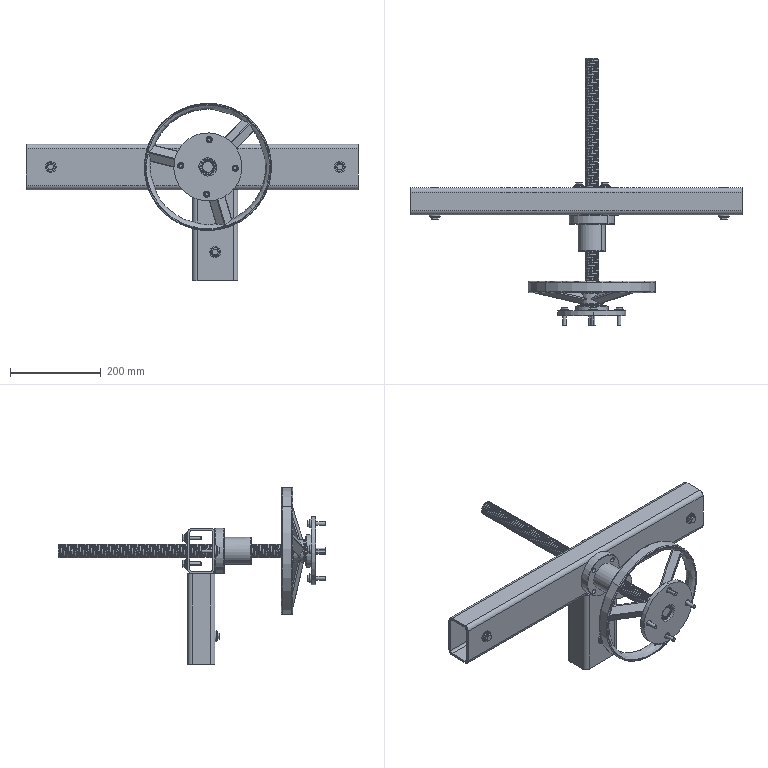Part | SolidWorks | 38 solids | 1047 faces | box 730 x 587.153 x 390 mm | volume 2603306 mm3 | cylinder 447 | plane 270 | cone 199 | spline 131 | commonest cylinder face diameters 30 x172 24 x40 12.9 x33 19.1 x33 14 x26 8 x24